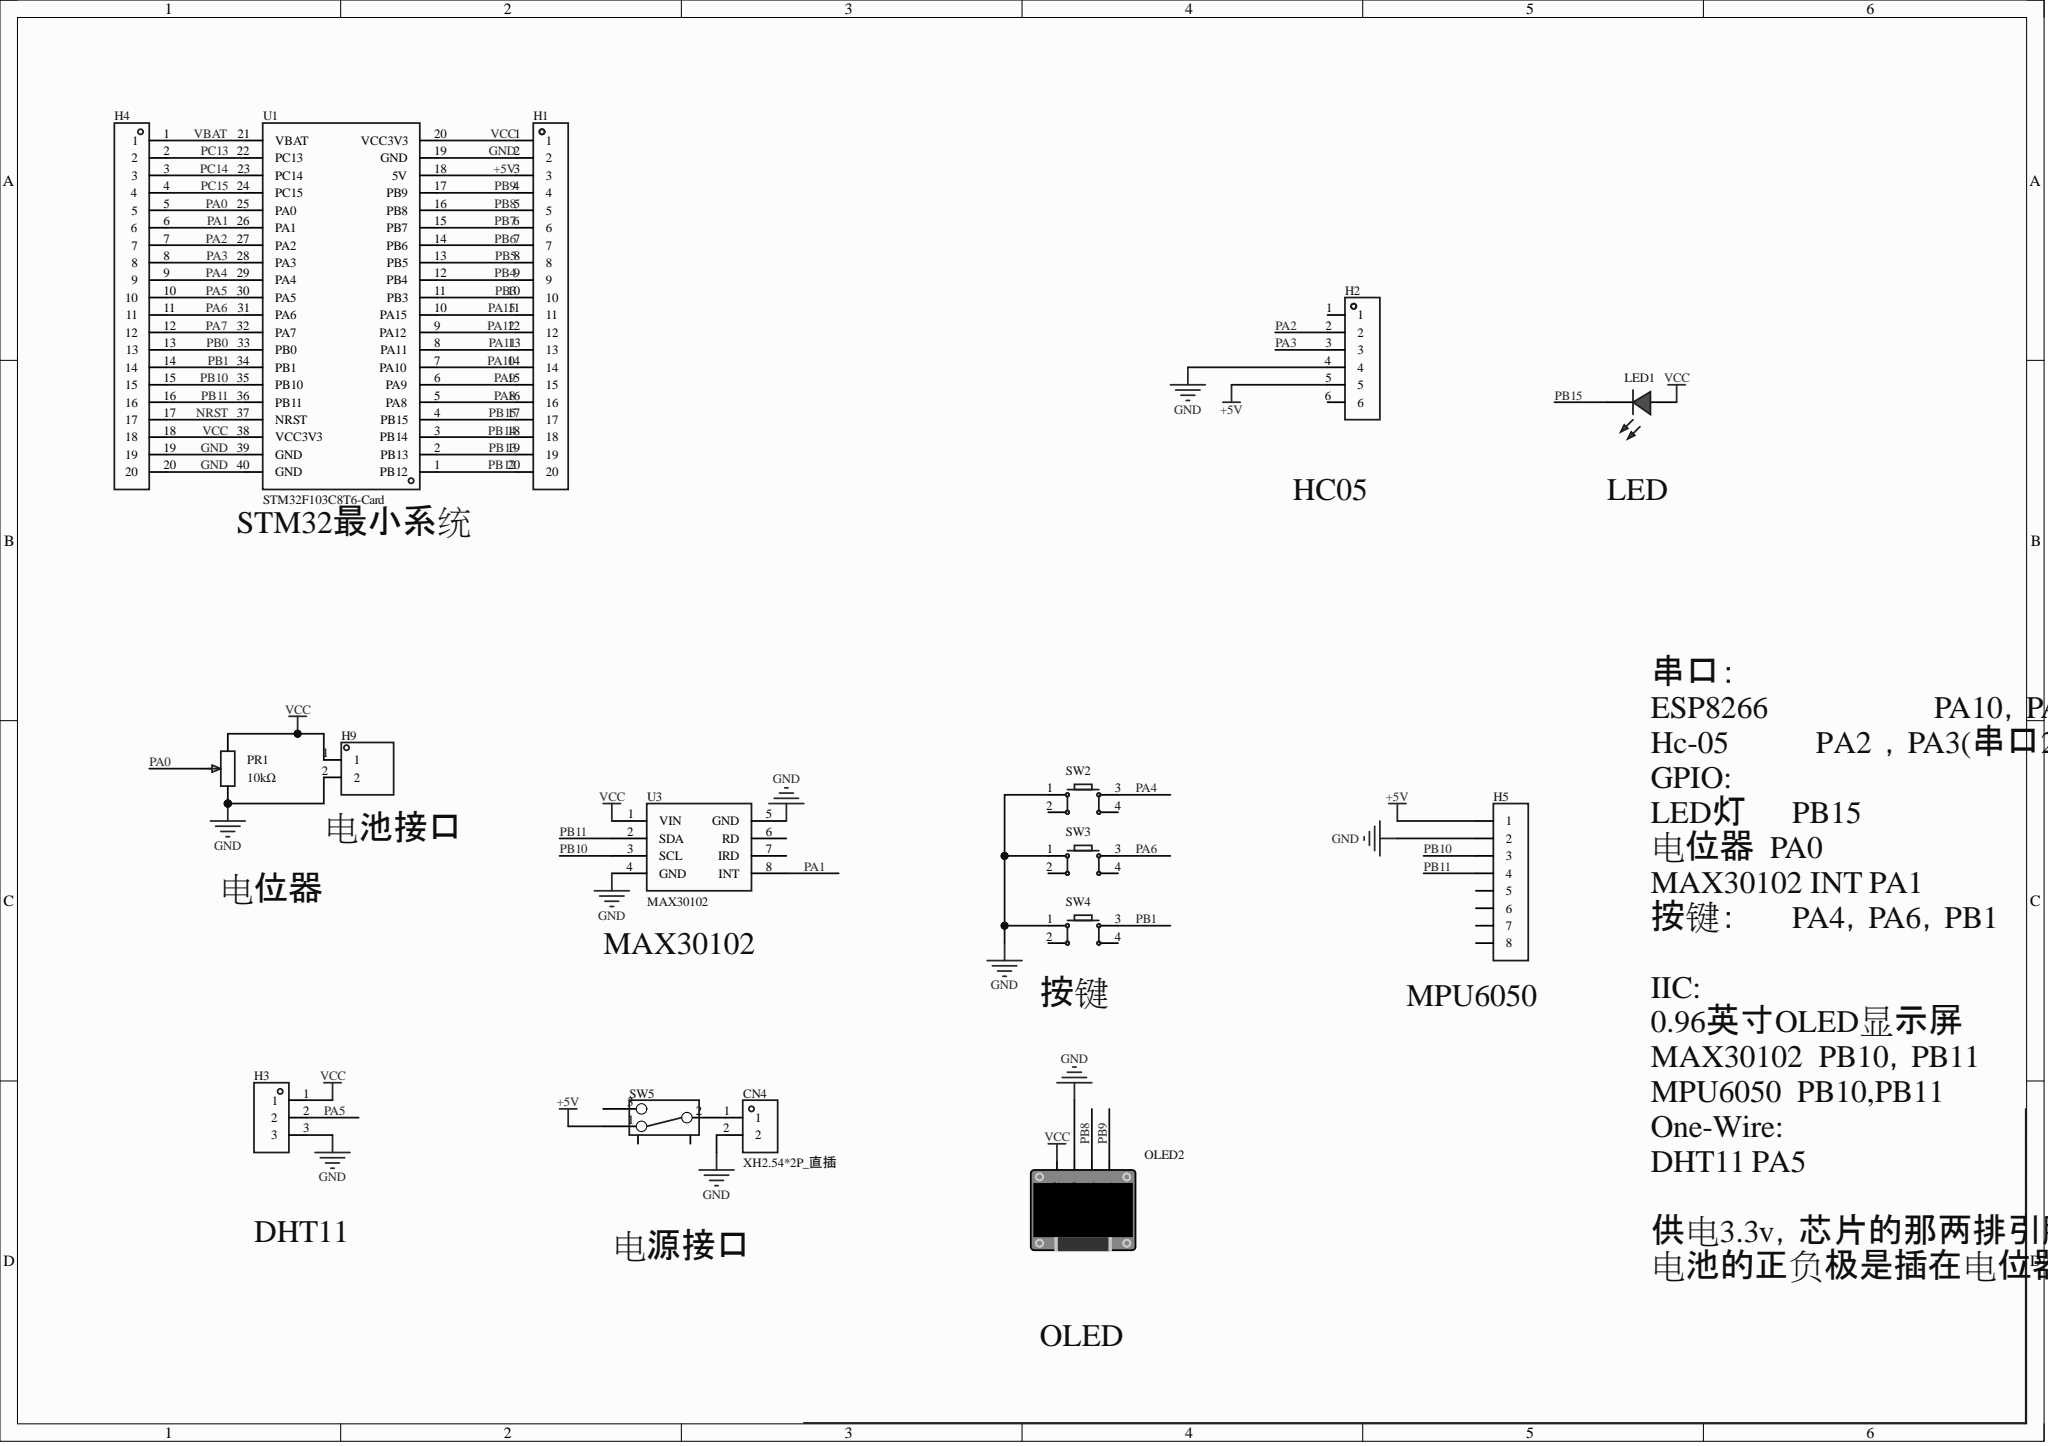Circuit board | Altium Designer | 16 parts | 38 nets
Bill of materials:
Comment,Description,Designator,Footprint,LibRef,Quantity
"XH2.54*2P_直插","","CN4","CONN-TH_2P-P2.50-XH2.54-2P","XH2.54*2P_直插","1"
"","间距:2.54mm;总PIN位数:20;排数:1;插针结构:-;行距:-;安装类型:直插;圆针/方针:-;额定电流:-;额定电压:-;配合针长度:-;塑高:-;触头材质:黄铜;触头镀层:-;颜色:黑色;","H1, H4","HDR-TH_20P-P2.54-V-M-1","HDR-M_2.54_1x20P","2"
"","","H2","HDR-TH_6P-P2.54-V-F","HDR-F_2.54_1x6P","1"
"","","H3","HDR-TH_3P-P2.54-V-F","HDR-F_2.54_1x3P","1"
"","","H5","HDR-TH_8P-P2.54-V-F-1","HDR-F_2.54_1x8P","1"
"","","H9","HDR-TH_2P-P2.54-V-M-1","HDR-M_2.54_1x2P","1"
"","","LED1","LED_TH-3mm","LED_TH-R_3mm","1"
"","","OLED2","0.96OLED_4P","0.96OLED模块_4P","1"
"10kΩ","","PR1","R_3296","R_3296","1"
"","","SW2, SW3, SW4","SW-TH_4P-L6.0-W6.0-P4.50-LS6.5","Key_TH_6x6x6","3"
"","","SW5","拨动开关","拨动开关_正","1"
"STM32F103C8T6-Card","","U1","CONN-TH_L53.3-W22.9_STM32F103C8T6-CARD","STM32F103C8T6-Card","1"
"MAX30102","","U3","MAX30102","MAX30102","1"
Netlist (Protel format):
[
CN4
CONN-TH_2P-P2.50-XH2.54-2P
XH2.54*2P_直插



]
[
H1
HDR-TH_20P-P2.54-V-M-1




]
[
H2
HDR-TH_6P-P2.54-V-F




]
[
H3
HDR-TH_3P-P2.54-V-F




]
[
H4
HDR-TH_20P-P2.54-V-M-1




]
[
H5
HDR-TH_8P-P2.54-V-F-1




]
[
H9
HDR-TH_2P-P2.54-V-M-1




]
[
LED1
LED_TH-3mm




]
[
OLED2
0.96OLED_4P




]
[
PR1
R_3296
10kΩ



]
[
SW2
SW-TH_4P-L6.0-W6.0-P4.50-LS6.5




]
[
SW3
SW-TH_4P-L6.0-W6.0-P4.50-LS6.5




]
[
SW4
SW-TH_4P-L6.0-W6.0-P4.50-LS6.5




]
[
SW5
拨动开关




]
[
U1
CONN-TH_L53.3-W22.9_STM32F103C8T6-CARD
STM32F103C8T6-Card



]
[
U3
MAX30102
MAX30102



]
(
VCC
H1-1
H3-1
H4-18
H9-1
LED1-1
OLED2-1
PR1-1
U1-20
U1-38
U3-1
)
(
VBAT
H4-1
U1-21
)
(
PC15
H4-4
U1-24
)
(
PC14
H4-3
U1-23
)
(
PC13
H4-2
U1-22
)
(
PB15
H1-17
LED1-2
U1-4
)
(
PB14
H1-18
U1-3
)
(
PB13
H1-19
U1-2
)
(
PB12
H1-20
U1-1
)
(
PB11
H4-16
H5-4
U1-36
U3-2
)
(
PB10
H4-15
H5-3
U1-35
U3-3
)
(
PB9
H1-4
OLED2-4
U1-17
)
(
PB8
H1-5
OLED2-3
U1-16
)
(
PB7
H1-6
U1-15
)
(
PB6
H1-7
U1-14
)
(
PB5
H1-8
U1-13
)
(
PB4
H1-9
U1-12
)
(
PB3
H1-10
U1-11
)
(
PB1
H4-14
SW4-3
U1-34
)
(
PB0
H4-13
U1-33
)
(
PA15
H1-11
U1-10
)
(
PA12
H1-12
U1-9
)
(
PA11
H1-13
U1-8
)
(
PA10
H1-14
U1-7
)
(
PA9
H1-15
U1-6
)
(
PA8
H1-16
U1-5
)
(
PA7
H4-12
U1-32
)
(
PA6
H4-11
SW3-3
U1-31
)
(
PA5
H3-2
H4-10
U1-30
)
(
PA4
H4-9
SW2-3
U1-29
)
(
PA3
H2-3
H4-8
U1-28
)
(
PA2
H2-2
H4-7
U1-27
)
(
PA1
H4-6
U1-26
U3-8
)
(
PA0
H4-5
PR1-2
U1-25
)
(
NRST
H4-17
U1-37
)
(
NetCN4_1
CN4-1
SW5-2
)
(
GND
CN4-2
H1-2
H2-4
H3-3
H4-19
H4-20
H5-2
H9-2
OLED2-2
PR1-3
SW2-1
SW3-1
SW4-1
U1-19
U1-39
U1-40
U3-4
U3-5
)
(
+5V
H1-3
H2-5
H5-1
SW5-1
U1-18
)